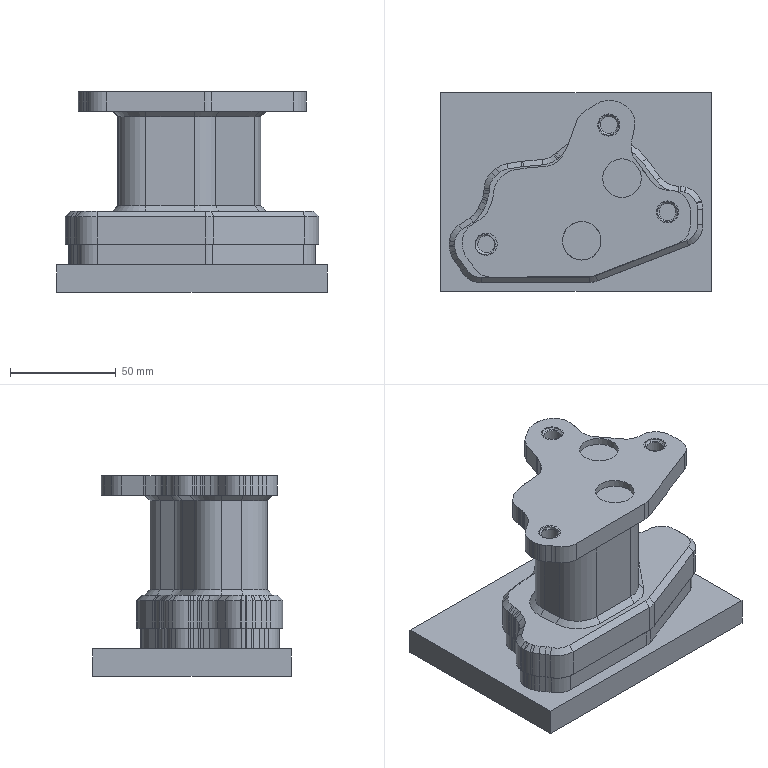NC program | NX | posted by the shop | part box 128.162 x 94.109 x 95 mm
Lines 1 to 907 of 131503:
1 BEGIN PGM A MM
2 BLK FORM 0.1 Z X-200 Y-200 Z-20
3 BLK FORM 0.2  X+200  Y+200  Z+0
4 CYCL DEF 247 DATUM SETTING ~
Q339=+1
5 * - OPERATION: 动态开粗_COPY - TOOL: T17 C-D20
6 M5
7 M9
8 PLANE RESET STAY
9 CALL LBL100
10 ;(C-D20 D=20. R=0.)
11 M01
12 TOOL CALL 17 Z S5500
13 CALL LBL101
14 M3 M8
15 M51
16 CYCL DEF 7.0
17 CYCL DEF 7.1 X0
18 CYCL DEF 7.2 Y0
19 CYCL DEF 7.3 Z0
20 CYCL DEF 32.0 TOLERANCE
21 CYCL DEF 32.1 T0.096
22 CYCL DEF 32.2 HSC-MODE:0
23 L M126
24 L A+0.0 C+0.0 FMAX
25 L X-64.6381 Y-62.2688 FMAX
26 L Z5.6 FMAX
27 L Z-41.4 FMAX
28 L Z-44.4 F4000.
29 L X-65.2249 Y-58.6321
30 CC X-67.2211 Y-58.9557
31 C X-66.6876 Y-57.005 DR+
32 CC X-63.5608 Y-44.6263
33 C X-75.0894 Y-50.1127 DR-
34 CC X-50.9463 Y-38.6348
35 C X-77.6301 Y-40.2486 DR-
36 CC X129.1158 Y-26.3608
37 C X-78.0747 Y-23.3848 DR-
38 L X-78.046 Y43.4708
39 CC X-66.5594 Y42.2154
40 C X-73.4593 Y51.4841 DR-
41 CC X-81.0452 Y57.4973
42 C X-72.4257 Y53.0917 DR+
43 CC X-63.9857 Y46.8105
44 C X-66.5375 Y57.0172 DR-
45 CC X-66.994 Y58.9644
46 C X-67.3023 Y60.9405 DR+
47 L X-67.7443 Y60.8715
48 L X-71.6615 Y60.2602 Z-43.9
49 L X-74.0482 Y59.8878 F15000.
50 CC X-73.7265 Y57.8856
51 C X-75.154 Y59.3259 DR+
52 L X-82.9516 Y51.5284
53 CC X-77.8446 Y46.4233
54 C X-85.0656 Y46.4246 DR+
55 L Y-25.4627
56 CC X15.891 Y-25.4556
57 C X-83.3393 Y-44.0456 DR+
58 L X-82.356 Y-49.2923
59 CC X-69.1974 Y-46.8244
60 C X-78.8027 Y-56.1505 DR+
61 L X-75.8842 Y-59.1556
62 CC X-74.4382 Y-57.7401
63 C X-74.7351 Y-59.7417 DR+
64 L X-71.9244 Y-60.1472
65 L X-70.0495 Y-60.4256 Z-44.1391 F4000.
66 L X-68.1703 Y-60.6737 Z-44.3782
67 L X-67.9978 Y-60.6835 Z-44.4
68 CC X-68.0574 Y-58.6844
69 C X-67.2677 Y-56.8468 DR+
70 CC X-63.9193 Y-46.8931
71 C X-73.873 Y-50.2416 DR-
72 CC X-32.3004 Y-34.5195
73 C X-76.7096 Y-36.3333 DR-
74 CC X259.3441 Y-20.2611
75 C X-77.0763 Y-16.8399 DR-
76 L X-77.0385 Y39.5418
77 CC X-57.875 Y37.4408
78 C X-74.5031 Y47.1958 DR-
79 CC X-93.6033 Y51.8201
80 C X-74.0913 Y49.4785 DR+
81 CC X-64.3957 Y46.985
82 C X-73.0825 Y51.9611 DR-
83 CC X-74.8273 Y52.9389
84 C X-74.8609 Y54.9387 DR+
85 CC X-74.7828 Y52.7966
86 CP IPA39.8769 IZ.1881 DR+
87 L X-78.155 Y52.8585 Z-43.9
88 L X-79.1315 Y52.0981 F15000.
89 L X-80.0829 Y51.3065
90 CC X-78.6074 Y49.9349
91 C X-80.6219 Y49.9409 DR+
92 L X-80.6327 Y-46.3389
93 CC X-78.5897 Y-46.3266
94 C X-80.3179 Y-47.4161 DR+
95 L X-79.1856 Y-49.188
96 L X-78.2717 Y-50.635 Z-44.116 F4000.
97 L X-77.3271 Y-52.0622 Z-44.3319
98 L X-76.9257 Y-52.4226 Z-44.4
99 CC X-75.8026 Y-50.7677
100 C X-73.873 Y-50.2416 DR+
101 CC X-55.3891 Y-45.2768
102 C X-74.4854 Y-46.5552 DR-
103 CC X78.9759 Y-24.6557
104 C X-76.0352 Y-23.4267 DR-
105 L X-76.0582 Y35.6979
106 CC X-44.9209 Y33.8344
107 C X-74.4274 Y43.9524 DR-
108 L X-74.3565 Y47.7592
109 CC X-76.3567 Y47.7861
110 C X-76.5758 Y49.7745 DR+
111 CC X-76.3099 Y47.6971
112 CP IPA51.5204 IZ.2375 DR+
113 L X-79.2965 Y47.0806 Z-43.9
114 L X-80.7527 Y45.0077 F15000.
115 CC X-79.0849 Y43.8481
116 C X-81.1162 Y43.8565 DR+
117 L X-81.0479 Y-44.3701
118 CC X-79.0136 Y-44.3579
119 C X-80.6972 Y-45.4998 DR+
120 L X-79.3207 Y-47.5066
121 L X-78.5503 Y-48.6479 Z-44.0738 F4000.
122 L X-77.7443 Y-49.7644 Z-44.2477
123 CC X-76.2434 Y-48.3254
124 CP IPA33.3004 IZ-.1523 DR+
125 CC X-76.2845 Y-48.3972
126 C X-74.2882 Y-48.2728 DR+
127 CC X26.3005 Y-43.293
128 C X-74.3991 Y-41.7213 DR-
129 CC X483.5474 Y-13.8433
130 C X-75.0754 Y-9.1457 DR-
131 L X-75.0405 Y33.1679
132 CC X-28.9846 Y30.8517
133 C X-74.3801 Y38.9614 DR-
134 L Y44.3364
135 CC X-76.3801 Y44.3363
136 C X-78.2435 Y45.0628 DR+
137 L X-79.3058 Y41.2435 Z-43.9
138 L X-79.609 Y40.1683 F15000.
139 L X-79.8813 Y39.0849
140 L X-79.8993 Y38.8171
141 L Y-36.9087
142 L X-79.8276 Y-37.4395
143 L X-79.343 Y-39.1999
144 L X-78.2898 Y-43.022 Z-44.4 F4000.
145 CC X-76.3801 Y-42.4279
146 C X-74.3801 Y-42.428 DR+
147 L Y39.072
148 CC X-76.401 Y39.0713
149 C X-76.0188 Y41.0557 DR+
150 L X-79.1882 Y41.6649
151 CC X-79.5695 Y39.6812
152 C X-79.3149 Y37.6773 DR+
153 L Z-41.4
154 L Z5.6 FMAX
155 L X-64.6381 Y-62.2688 FMAX
156 L Z-78.7 FMAX
157 L Z-81.7
158 L X-65.2249 Y-58.6321
159 CC X-67.2211 Y-58.9557
160 C X-66.6876 Y-57.005 DR+
161 CC X-63.5608 Y-44.6263
162 C X-75.0894 Y-50.1127 DR-
163 CC X-50.9463 Y-38.6348
164 C X-77.6301 Y-40.2486 DR-
165 CC X129.1158 Y-26.3608
166 C X-78.0747 Y-23.3848 DR-
167 L X-78.046 Y43.4708
168 CC X-66.5594 Y42.2154
169 C X-73.4593 Y51.4841 DR-
170 CC X-81.0452 Y57.4973
171 C X-72.4257 Y53.0917 DR+
172 CC X-63.9857 Y46.8105
173 C X-66.5375 Y57.0172 DR-
174 CC X-66.994 Y58.9644
175 C X-67.3023 Y60.9405 DR+
176 L X-67.7443 Y60.8715
177 L X-71.6615 Y60.2602 Z-81.2
178 L X-74.0482 Y59.8878 F15000.
179 CC X-73.7265 Y57.8856
180 C X-75.154 Y59.3259 DR+
181 L X-82.9516 Y51.5284
182 CC X-77.8446 Y46.4233
183 C X-85.0656 Y46.4246 DR+
184 L Y-25.4627
185 CC X15.891 Y-25.4556
186 C X-83.3393 Y-44.0456 DR+
187 L X-82.356 Y-49.2923
188 CC X-69.1974 Y-46.8244
189 C X-78.8027 Y-56.1505 DR+
190 L X-75.8842 Y-59.1556
191 CC X-74.4382 Y-57.7401
192 C X-74.7351 Y-59.7417 DR+
193 L X-71.9244 Y-60.1472
194 L X-70.0495 Y-60.4256 Z-81.4391 F4000.
195 L X-68.1703 Y-60.6737 Z-81.6782
196 L X-67.9978 Y-60.6835 Z-81.7
197 CC X-68.0574 Y-58.6844
198 C X-67.2677 Y-56.8468 DR+
199 CC X-63.9193 Y-46.8931
200 C X-73.873 Y-50.2416 DR-
201 CC X-32.3004 Y-34.5195
202 C X-76.7096 Y-36.3333 DR-
203 CC X259.3441 Y-20.2611
204 C X-77.0763 Y-16.8399 DR-
205 L X-77.0385 Y39.5418
206 CC X-57.875 Y37.4408
207 C X-74.5031 Y47.1958 DR-
208 CC X-93.6033 Y51.8201
209 C X-74.0913 Y49.4785 DR+
210 CC X-64.3957 Y46.985
211 C X-73.0825 Y51.9611 DR-
212 CC X-74.8273 Y52.9389
213 C X-74.8609 Y54.9387 DR+
214 CC X-74.7828 Y52.7966
215 CP IPA39.8769 IZ.1881 DR+
216 L X-78.155 Y52.8585 Z-81.2
217 L X-79.1315 Y52.0981 F15000.
218 L X-80.0829 Y51.3065
219 CC X-78.6074 Y49.9349
220 C X-80.6219 Y49.9409 DR+
221 L X-80.6327 Y-46.3389
222 CC X-78.5897 Y-46.3266
223 C X-80.3179 Y-47.4161 DR+
224 L X-79.1856 Y-49.188
225 L X-78.2717 Y-50.635 Z-81.416 F4000.
226 L X-77.3271 Y-52.0622 Z-81.6319
227 L X-76.9257 Y-52.4226 Z-81.7
228 CC X-75.8026 Y-50.7677
229 C X-73.873 Y-50.2416 DR+
230 CC X-55.3891 Y-45.2768
231 C X-74.4854 Y-46.5552 DR-
232 CC X78.9759 Y-24.6557
233 C X-76.0352 Y-23.4267 DR-
234 L X-76.0582 Y35.6979
235 CC X-44.9209 Y33.8344
236 C X-74.4274 Y43.9524 DR-
237 L X-74.3565 Y47.7592
238 CC X-76.3567 Y47.7861
239 C X-76.5758 Y49.7745 DR+
240 CC X-76.3099 Y47.6971
241 CP IPA51.5204 IZ.2375 DR+
242 L X-79.2965 Y47.0806 Z-81.2
243 L X-80.7527 Y45.0077 F15000.
244 CC X-79.0849 Y43.8481
245 C X-81.1162 Y43.8565 DR+
246 L X-81.0479 Y-44.3701
247 CC X-79.0136 Y-44.3579
248 C X-80.6972 Y-45.4998 DR+
249 L X-79.3207 Y-47.5066
250 L X-78.5503 Y-48.6479 Z-81.3738 F4000.
251 L X-77.7443 Y-49.7644 Z-81.5477
252 CC X-76.2434 Y-48.3254
253 CP IPA33.3004 IZ-.1523 DR+
254 CC X-76.2845 Y-48.3972
255 C X-74.2882 Y-48.2728 DR+
256 CC X26.3006 Y-43.293
257 C X-74.3991 Y-41.7213 DR-
258 CC X483.5474 Y-13.8433
259 C X-75.0754 Y-9.1457 DR-
260 L X-75.0405 Y33.1679
261 CC X-28.9846 Y30.8517
262 C X-74.3801 Y38.9614 DR-
263 L Y44.3364
264 CC X-76.3801 Y44.3363
265 C X-78.2435 Y45.0628 DR+
266 L X-79.3058 Y41.2435 Z-81.2
267 L X-79.609 Y40.1683 F15000.
268 L X-79.8813 Y39.0849
269 L X-79.8993 Y38.8171
270 L Y-36.9087
271 L X-79.8276 Y-37.4395
272 L X-79.343 Y-39.1999
273 L X-78.2898 Y-43.022 Z-81.7 F4000.
274 CC X-76.3801 Y-42.4279
275 C X-74.3801 Y-42.428 DR+
276 L Y39.072
277 CC X-76.401 Y39.0713
278 C X-76.0188 Y41.0557 DR+
279 L X-79.1882 Y41.6649
280 CC X-79.5695 Y39.6812
281 C X-79.3149 Y37.6773 DR+
282 L Z-78.7
283 L Z5.6 FMAX
284 L X62.5938 Y62.3089 FMAX
285 L Z-41.4 FMAX
286 L Z-44.4
287 CC X62.6738 Y60.2896
288 C X64.6499 Y60.7124 DR-
289 L X65.1088 Y58.5642
290 CC X67.0859 Y58.9878
291 C X66.7119 Y57.0007 DR+
292 CC X63.4656 Y44.5388
293 C X75.1287 Y49.9985 DR-
294 CC X50.4575 Y38.4647
295 C X77.6487 Y39.9932 DR-
296 CC X-132.8635 Y26.3435
297 C X78.0733 Y23.6284 DR-
298 L X78.0464 Y-43.4545
299 CC X66.5542 Y-42.2325
300 C X73.4839 Y-51.4815 DR-
301 L X71.9663 Y-53.6802
302 CC X62.8803 Y-45.5088
303 C X68.5579 Y-56.3297 DR-
304 L X66.7172 Y-57.0079
305 CC X67.2019 Y-58.9502
306 C X67.6274 Y-60.9064 DR+
307 L X71.5448 Y-60.2964 Z-43.9
308 L X74.2272 Y-59.8787 F15000.
309 CC X73.9063 Y-57.8764
310 C X75.3337 Y-59.3167 DR+
311 L X83.1313 Y-51.5192
312 CC X78.0243 Y-46.4141
313 C X85.2453 Y-46.4154 DR+
314 L Y25.5025
315 CC X-12.8027 Y25.4957
316 C X83.4802 Y44.0164 DR+
317 L X82.4553 Y49.3429
318 CC X70.0761 Y46.9591
319 C X78.925 Y55.9381 DR+
320 L X75.572 Y59.2417
321 CC X74.1549 Y57.7902
322 C X74.4684 Y59.7944 DR+
323 L X71.7716 Y60.2035
324 L X67.8514 Y60.7952 Z-44.4 F4000.
325 CC X67.661 Y58.8043
326 C X66.9555 Y56.9329 DR+
327 CC X63.9621 Y46.9025
328 C X73.7629 Y50.5783 DR-
329 CC X31.4752 Y34.3855
330 C X76.7259 Y36.0708 DR-
331 CC X-272.8684 Y20.0983
332 C X77.0752 Y16.8268 DR-
333 L X77.0473 Y-39.4006
334 CC X57.7068 Y-37.4513
335 C X74.4658 Y-47.2998 DR-
336 CC X79.0145 Y-48.6425
337 C X74.2732 Y-48.5223 DR+
338 CC X63.5123 Y-46.8644
339 C X73.1423 Y-51.9446 DR-
340 CC X74.9604 Y-52.7786
341 C X74.7473 Y-54.7674 DR+
342 CC X74.9365 Y-52.6722
343 CP IPA46.4743 IZ.2151 DR+
344 L X78.1168 Y-52.8805 Z-43.9
345 L X79.1344 Y-52.1132 F15000.
346 L X80.1259 Y-51.3124
347 CC X78.6684 Y-49.9233
348 C X80.6818 Y-49.9244 DR+
349 L X80.4755 Y46.7914
350 CC X78.4306 Y46.7741
351 C X80.1648 Y47.8577 DR+
352 L X79.1147 Y49.5148
353 L X77.2267 Y52.4725 Z-44.3428 F4000.
354 L X76.9202 Y52.8069 Z-44.4
355 CC X75.628 Y51.2803
356 C X73.7158 Y50.6941 DR+
357 CC X56.9761 Y45.3618
358 C X74.5117 Y46.4364 DR-
359 CC X-82.3019 Y24.4596
360 C X76.0379 Y23.0517 DR-
361 L X76.0526 Y-35.8229
362 CC X44.5148 Y-33.7783
363 C X74.415 Y-44.015 DR-
364 L X74.3105 Y-47.9258
365 CC X76.3069 Y-48.0502
366 C X76.664 Y-50.0183 DR+
367 CC X76.2558 Y-47.9616
368 CP IPA48.1212 IZ.222 DR+
369 L X79.305 Y-47.2152 Z-43.9
370 L X80.1055 Y-46.0667 F15000.
371 L X80.8701 Y-44.894
372 L X81.0159 Y-44.469
373 L X81.0702 Y-44.0231
374 L X81.1135 Y43.8565
375 CC X79.082 Y43.8475
376 C X80.7506 Y45.0063 DR+
377 L X79.3324 Y47.0274
378 L X77.8867 Y49.0644 Z-44.2154 F4000.
379 CC X76.3416 Y47.788
380 CP IPA41.8361 IZ-.1846 DR+
381 CC X76.3539 Y47.7901
382 C X74.3538 Y47.7592 DR+
383 CC X359.4998 Y48.4494
384 C X74.8188 Y32.1579 DR+
385 CC X-816.6851 Y9.671
386 C X75.0767 Y2.9105 DR-
387 L X75.0408 Y-33.1515
388 CC X31.263 Y-31.0727
389 C X74.3807 Y-38.9263 DR-
390 L Y-44.3013
391 CC X76.3807 Y-44.3013
392 C X78.2705 Y-44.9561 DR+
393 L X79.3267 Y-41.1348 Z-43.9
394 L X79.6191 Y-40.0963 F15000.
395 L X79.8819 Y-39.0499
396 L X79.8999 Y-38.7821
397 L Y36.8956
398 L X79.8282 Y37.4264
399 L X79.3211 Y39.2688
400 L X78.2634 Y43.0896 Z-44.4 F4000.
401 CC X76.3807 Y42.4148
402 C X74.3807 Y42.4149 DR+
403 L Y-38.9601
404 CC X76.401 Y-38.9598
405 C X76.6988 Y-40.958 DR+
406 L X79.3347 Y-40.5647
407 L Z-41.4
408 L Z5.6 FMAX
409 L X62.5938 Y62.3089 FMAX
410 L Z-78.7 FMAX
411 L Z-81.7
412 CC X62.6738 Y60.2896
413 C X64.6474 Y60.724 DR-
414 L X65.125 Y58.55
415 CC X67.0998 Y58.9853
416 C X66.7119 Y57.0007 DR+
417 CC X63.4656 Y44.5388
418 C X75.1287 Y49.9985 DR-
419 CC X50.4575 Y38.4647
420 C X77.6487 Y39.9932 DR-
421 CC X-132.8635 Y26.3435
422 C X78.0733 Y23.6284 DR-
423 L X78.0464 Y-43.4545
424 CC X66.5542 Y-42.2325
425 C X73.4839 Y-51.4815 DR-
426 L X71.9663 Y-53.6802
427 CC X62.8803 Y-45.5088
428 C X68.5579 Y-56.3297 DR-
429 L X66.7172 Y-57.0079
430 CC X67.2019 Y-58.9502
431 C X67.6274 Y-60.9064 DR+
432 L X71.5448 Y-60.2964 Z-81.2
433 L X74.2272 Y-59.8787 F15000.
434 CC X73.9063 Y-57.8764
435 C X75.3337 Y-59.3167 DR+
436 L X83.1313 Y-51.5192
437 CC X78.0243 Y-46.4141
438 C X85.2453 Y-46.4154 DR+
439 L Y25.5025
440 CC X-12.8027 Y25.4957
441 C X83.4802 Y44.0164 DR+
442 L X82.4553 Y49.3429
443 CC X70.0761 Y46.9591
444 C X78.925 Y55.9381 DR+
445 L X75.572 Y59.2417
446 CC X74.1549 Y57.7902
447 C X74.4684 Y59.7944 DR+
448 L X71.7716 Y60.2035
449 L X67.8514 Y60.7952 Z-81.7 F4000.
450 CC X67.661 Y58.8043
451 C X66.9555 Y56.9329 DR+
452 CC X63.9621 Y46.9025
453 C X73.7629 Y50.5783 DR-
454 CC X31.4752 Y34.3855
455 C X76.7259 Y36.0708 DR-
456 CC X-272.8684 Y20.0983
457 C X77.0752 Y16.8268 DR-
458 L X77.0473 Y-39.4006
459 CC X57.7068 Y-37.4513
460 C X74.4658 Y-47.2998 DR-
461 CC X79.0145 Y-48.6425
462 C X74.2732 Y-48.5223 DR+
463 CC X63.5123 Y-46.8644
464 C X73.1423 Y-51.9446 DR-
465 CC X74.9604 Y-52.7786
466 C X74.7473 Y-54.7674 DR+
467 CC X74.9365 Y-52.6722
468 CP IPA46.4743 IZ.2151 DR+
469 L X78.1168 Y-52.8805 Z-81.2
470 L X79.1344 Y-52.1132 F15000.
471 L X80.1259 Y-51.3124
472 CC X78.6684 Y-49.9233
473 C X80.6818 Y-49.9244 DR+
474 L X80.4755 Y46.7914
475 CC X78.4306 Y46.7741
476 C X80.1648 Y47.8577 DR+
477 L X79.1147 Y49.5148
478 L X77.2267 Y52.4725 Z-81.6428 F4000.
479 L X76.9202 Y52.8069 Z-81.7
480 CC X75.628 Y51.2803
481 C X73.7158 Y50.6941 DR+
482 CC X56.9761 Y45.3618
483 C X74.5117 Y46.4364 DR-
484 CC X-82.3019 Y24.4596
485 C X76.0379 Y23.0517 DR-
486 L X76.0526 Y-35.8229
487 CC X44.5148 Y-33.7783
488 C X74.415 Y-44.015 DR-
489 L X74.3105 Y-47.9258
490 CC X76.3069 Y-48.0502
491 C X76.664 Y-50.0183 DR+
492 CC X76.2558 Y-47.9616
493 CP IPA48.1212 IZ.222 DR+
494 L X79.305 Y-47.2152 Z-81.2
495 L X80.1055 Y-46.0667 F15000.
496 L X80.8701 Y-44.894
497 L X81.0159 Y-44.469
498 L X81.0702 Y-44.0231
499 L X81.1135 Y43.8565
500 CC X79.082 Y43.8475
501 C X80.7506 Y45.0063 DR+
502 L X79.3324 Y47.0274
503 L X77.8867 Y49.0644 Z-81.5154 F4000.
504 CC X76.3416 Y47.788
505 CP IPA41.8361 IZ-.1846 DR+
506 CC X76.3539 Y47.7901
507 C X74.3538 Y47.7592 DR+
508 CC X359.4999 Y48.4494
509 C X74.8188 Y32.1579 DR+
510 CC X-816.6851 Y9.671
511 C X75.0767 Y2.9105 DR-
512 L X75.0408 Y-33.1515
513 CC X31.263 Y-31.0727
514 C X74.3807 Y-38.9263 DR-
515 L Y-44.3013
516 CC X76.3807 Y-44.3013
517 C X78.2705 Y-44.9561 DR+
518 L X79.3267 Y-41.1348 Z-81.2
519 L X79.6191 Y-40.0963 F15000.
520 L X79.8819 Y-39.0499
521 L X79.8999 Y-38.7821
522 L Y36.8956
523 L X79.8282 Y37.4264
524 L X79.3211 Y39.2688
525 L X78.2634 Y43.0896 Z-81.7 F4000.
526 CC X76.3807 Y42.4148
527 C X74.3807 Y42.4149 DR+
528 L Y-38.9601
529 CC X76.401 Y-38.9598
530 C X76.6988 Y-40.958 DR+
531 L X79.3347 Y-40.5647
532 L Z-78.7
533 L Z5.6 FMAX
534 PLANE RESET STAY
535 * - OPERATION: 精飞平面 - TOOL: T17 C-D20
536 CYCL DEF 32.0 TOLERANCE
537 CYCL DEF 32.1 T0.036
538 CYCL DEF 32.2 HSC-MODE:0
539 L A+0.0 C+0.0 FMAX
540 L X76.2809 Y-40.7534 FMAX
541 L Z43. FMAX
542 L Z3.1 FMAX
543 L Z.1 F1500.
544 L X74.0809
545 L X-74.0809
546 L Y-24.452
547 L X74.0809
548 L Y-8.1507
549 L X-74.0809
550 L Y8.1507
551 L X74.0809
552 L Y24.452
553 L X-74.0809
554 L Y40.7534
555 L X74.0809
556 L X76.2809
557 L Z3.1
558 L Z43. FMAX
559 PLANE RESET STAY
560 * - OPERATION: 动态开粗 - TOOL: T17 C-D20
561 CYCL DEF 32.0 TOLERANCE
562 CYCL DEF 32.1 T0.096
563 CYCL DEF 32.2 HSC-MODE:0
564 L A+0.0 C+0.0 FMAX
565 L X-79.1931 Y-24.9744 FMAX
566 L Z5.6 FMAX
567 L Z-41.4 FMAX
568 L Z-44.4 F4000.
569 L X-76.8858 Y-26.1193
570 CC X-75.9882 Y-24.3093
571 C X-74.0804 Y-24.9744 DR+
572 CC X-103.6147 Y-17.8744
573 C X-73.2393 Y-17.7376 DR+
574 CC X-767.6787 Y-2.7045
575 C X-73.0802 Y-.4558 DR+
576 L X-73.0461 Y43.4708
577 CC X-61.3176 Y42.1555
578 C X-67.363 Y52.2917 DR-
579 CC X-55.5707 Y32.5157
580 C X-57.5748 Y55.4532 DR-
581 CC X-45.0783 Y-76.5411
582 C X-43.3441 Y56.0321 DR-
583 L X60.4448 Y56.0206
584 CC X59.2035 Y44.4007
585 C X69.1338 Y50.5612 DR-
586 CC X49.7352 Y38.5467
587 C X72.4633 Y40.5691 DR-
588 CC X-57.4553 Y27.9966
589 C X73.058 Y26.2144 DR-
590 L X73.0458 Y-43.4545
591 CC X61.4086 Y-42.1991
592 C X67.4768 Y-52.208 DR-
593 CC X55.6256 Y-32.7006
594 C X57.71 Y-55.4305 DR-
595 CC X45.0627 Y74.1115
596 C X43.2308 Y-56.0335 DR-
597 L X-60.6053 Y-56.014
598 CC X-59.2123 Y-44.3836
599 C X-69.1658 Y-50.5589 DR-
600 CC X-49.87 Y-38.6409
601 C X-72.4571 Y-40.6881 DR-
602 CC X8.786 Y-31.2452
603 C X-72.5692 Y-22.822 DR-
604 CC X-387.5348 Y-5.2348
605 C X-72.0878 Y-2.8148 DR+
606 L X-72.0491 Y39.4175
607 CC X-57.4642 Y38.2757
608 C X-64.4942 Y51.1054 DR-
609 CC X-51.0693 Y26.4223
610 C X-53.3108 Y54.4305 DR-
611 CC X-39.0488 Y-108.9859
612 C X-36.8296 Y55.0367 DR-
613 L X56.3912 Y55.0229
614 CC X55.2639 Y40.4088
615 C X68.1102 Y47.467 DR-
616 CC X43.4345 Y34.0086
617 C X71.4496 Y36.2827 DR-
618 CC X-79.1815 Y22.6646
619 C X72.0553 Y21.0518 DR-
620 L X72.0402 Y-39.5255
621 CC X57.4537 Y-38.2618
622 C X64.4734 Y-51.1104 DR-
623 CC X51.0351 Y-26.3439
624 C X53.2772 Y-54.4319 DR-
625 CC X39.2625 Y104.7801
626 C X37.296 Y-55.0355 DR-
627 L X-56.4266 Y-55.0241
628 CC X-55.2981 Y-40.4413
629 C X-68.1338 Y-47.4539 DR-
630 CC X-43.8328 Y-34.1812
631 C X-71.4123 Y-36.6461 DR-
632 CC X-4.493 Y-29.5245
633 C X-71.6233 Y-24.7892 DR-
634 CC X-660.7992 Y1.1722
635 C X-71.0761 Y6.5373 DR+
636 L X-71.0451 Y36.0373
637 CC X-54.4393 Y35.2875
638 C X-61.8862 Y50.1488 DR-
639 CC X-47.5727 Y21.3661
640 C X-50.0248 Y53.4178 DR-
641 CC X-35.091 Y-123.7813
642 C X-33.043 Y54.0341 DR-
643 L X52.8317 Y54.0264
644 CC X52.2865 Y37.3989
645 C X67.1224 Y44.9265 DR-
646 CC X38.5947 Y30.5765
647 C X70.4302 Y33.0774 DR-
648 CC X-112.4859 Y17.634
649 C X71.0634 Y15.0964 DR-
650 L X71.0493 Y-35.9032
651 CC X54.4523 Y-35.2873
652 C X61.981 Y-50.0913 DR-
653 CC X47.7926 Y-22.0839
654 C X50.5122 Y-53.3622 DR-
655 CC X35.214 Y116.0301
656 C X32.9087 Y-54.036 DR-
657 L X-53.0907 Y-54.0172
658 CC X-52.3018 Y-37.4024
659 C X-67.1863 Y-44.8272 DR-
660 CC X-39.488 Y-31.0006
661 C X-70.427 Y-32.0735 DR-
662 CC X93.5889 Y-26.2135
663 C X-70.3363 Y-18.2102 DR-
664 CC X-979.1699 Y4.5471
665 C X-70.0784 Y11.5402 DR+
666 CC X878.9921 Y19.8935
667 C X-70.017 Y33.542 DR-
668 CC X-51.896 Y32.7543
669 C X-59.6515 Y49.1507 DR-
670 CC X-44.5708 Y16.9764
671 C X-47.1445 Y52.4163 DR-
672 CC X-31.3648 Y-144.4649
673 C X-29.1619 Y53.0354 DR-
674 L X11.9637 Y53.0668
675 CC X16.3169 Y22.3388
676 C X19.2858 Y53.2313 DR-
677 CC X39.7258 Y1015.9654
678 C X48.0157 Y53.0501 DR+
679 CC X49.0523 Y32.1833
680 C X58.0821 Y51.0237 DR-
681 CC X48.7082 Y33.83
682 C X67.1145 Y40.5158 DR-
683 CC X26.0842 Y25.7234
684 C X69.6606 Y27.5658 DR-
685 CC X-312.1338 Y9.0746
686 C X70.0754 Y4.0737 DR-
687 L X70.0352 Y-33.1511
688 CC X51.8548 Y-32.7196
689 C X59.5761 Y-49.1846 DR-
690 CC X44.6091 Y-17.0786
691 C X47.301 Y-52.3994 DR-
692 CC X31.8843 Y132.6011
693 C X30.0693 Y-53.0318 DR-
694 L X-49.9274 Y-53.0206
695 CC X-49.7066 Y-34.7688
696 C X-66.3742 Y-42.2099 DR-
697 CC X-36.1997 Y-28.7343
698 C X-69.2273 Y-29.8595 DR-
699 CC X133.6335 Y-22.0111
700 C X-69.2465 Y-14.6742 DR-
701 CC X-1025.6017 Y4.9783
702 C X-69.0744 Y12.5366 DR+
703 CC X521.0636 Y19.29
704 C X-68.9911 Y31.2855 DR-
705 CC X-49.6782 Y30.5206
706 C X-57.8073 Y48.056 DR-
707 CC X-42.2199 Y14.1798
708 C X-45.1736 Y51.3529 DR-
709 CC X-28.4949 Y-148.0887
710 C X-26.0686 Y52.0344 DR-
711 L X7.8899 Y52.0739
712 CC X15.9792 Y27.7752
713 C X21.8989 Y52.6915 DR-
714 CC X33.1331 Y154.3707
715 C X34.7141 Y52.085 DR+
716 CC X38.0217 Y-295.1394
717 C X48.6442 Y51.9382 DR-
718 CC X47.5309 Y32.6196
719 C X65.1328 Y40.6585 DR-
720 CC X31.1758 Y25.1909
721 C X68.3639 Y28.2506 DR-
722 CC X-125.9894 Y11.6332
723 C X69.0588 Y9.2714 DR-
724 L X69.0487 Y-29.9783
725 CC X49.0081 Y-30.2354
726 C X64.8348 Y-42.5321 DR-
727 CC X47.435 Y-27.7197
728 C X53.3926 Y-49.7803 DR-
729 CC X38.1987 Y6.6141
730 C X39.4451 Y-51.7779 DR-
731 CC X20.2114 Y574.5371
732 C X14.9486 Y-52.051 DR-
733 L X-47.1761 Y-52.0192
734 CC X-47.3409 Y-32.2541
735 C X-60.274 Y-47.2015 DR-
736 CC X-44.5143 Y-30.4719
737 C X-66.9994 Y-35.2326 DR-
738 CC X-8.5947 Y-22.9533
739 C X-68.2655 Y-21.822 DR-
740 L X-68.0769 Y9.0483
741 CC X657.1293 Y15.8438
742 C X-67.9932 Y28.7917 DR-
743 CC X-47.5571 Y28.4043
744 C X-55.8405 Y47.0903 DR-
745 CC X-39.7648 Y10.5572
746 C X-42.8057 Y50.3548 DR-
747 CC X-25.1363 Y-171.8932
748 C X-22.2 Y51.0367 DR-
749 L X5.0633 Y51.0775
750 CC X4.7996 Y55.747
751 C X7.2432 Y51.7593 DR+
752 CC X12.7872 Y39.9081
753 C X10.6802 Y52.8211 DR-
754 L X12.4045 Y53.1495
755 CC X15.4854 Y30.3956
756 C X15.8431 Y53.3543 DR-
757 CC X16.2034 Y24.2804
758 C X19.2817 Y53.1932 DR-
759 CC X4.298 Y-23.1029
760 C X24.6658 Y51.9354 DR-
761 CC X35.4039 Y123.4693
762 C X35.9322 Y51.1359 DR+
763 CC X37.1619 Y-135.8876
764 C X47.0689 Y50.8774 DR-
765 CC X45.5095 Y30.6187
766 C X64.0193 Y38.9991 DR-
767 CC X28.4715 Y22.9741
768 C X67.328 Y26.2337 DR-
769 CC X-130.2771 Y9.0898
770 C X68.0565 Y6.7558 DR-
771 L X68.0503 Y-27.2766
772 CC X44.9804 Y-27.6813
773 C X65.3216 Y-38.5725 DR-
774 CC X46.5871 Y-27.3374
775 C X53.7818 Y-47.9638 DR-
776 CC X38.001 Y-2.6063
777 C X40.3297 Y-50.5741 DR-
778 CC X22.5364 Y272.2534
779 C X19.0892 Y-51.0457 DR-
780 L X-44.8027 Y-51.011
781 CC X-45.0324 Y-29.3289
782 C X-57.1793 Y-47.2905 DR-
783 CC X-43.8297 Y-29.4254
784 C X-65.3917 Y-35.1221 DR-
785 CC X-13.6363 Y-21.5389
786 C X-67.1443 Y-21.3984 DR-
787 CC X931.6977 Y-11.8259
788 C X-67.0883 Y2.4395 DR-
789 L X-67.033 Y25.5447
790 CC X-42.9122 Y25.7124
791 C X-64.0717 Y37.2931 DR-
792 CC X-44.7192 Y25.4395
793 C X-52.1104 Y46.8964 DR-
794 CC X-35.8548 Y-.3177
795 C X-38.2831 Y49.5573 DR-
796 CC X-19.6209 Y-291.8834
797 C X-15.6679 Y50.0441 DR-
798 CC X-9.1908 Y865.0086
799 C X3.0362 Y50.1101 DR+
800 CC X2.9206 Y54.4963
801 C X5.5273 Y50.9668 DR+
802 CC X14.8927 Y33.3841
803 C X12.4045 Y53.1495 DR-
804 CC X15.4854 Y30.3956
805 C X15.8431 Y53.3543 DR-
806 CC X16.2034 Y24.2804
807 C X19.2817 Y53.1932 DR-
808 CC X16.1462 Y30.6982
809 C X25.243 Y51.5093 DR-
810 CC X34.811 Y88.7469
811 C X34.335 Y50.3027 DR+
812 CC X27.9591 Y-256.8808
813 C X44.9517 Y49.8986 DR-
814 CC X43.5219 Y28.6496
815 C X63.047 Y37.1546 DR-
816 CC X25.2034 Y20.7212
817 C X66.3209 Y24.1182 DR-
818 CC X-132.9521 Y6.9399
819 C X67.0507 Y5.0149 DR-
820 L X67.0396 Y-25.2347
821 CC X42.1692 Y-25.5406
822 C X64.4002 Y-36.6947 DR-
823 CC X44.9576 Y-25.7352
824 C X52.604 Y-46.7032 DR-
825 CC X36.2885 Y-1.8815
826 C X38.9317 Y-49.5071 DR-
827 CC X20.6528 Y250.5199
828 C X17.1936 Y-50.0435 DR-
829 L X10.0251 Y-50.0748
830 CC X5.5372 Y-30.0926
831 C X5.5273 Y-50.5726 DR-
832 L X-40.8942 Y-50.7472
833 CC X-38.4651 Y-12.0939
834 C X-51.1196 Y-48.6978 DR-
835 CC X-43.2303 Y-28.8063
836 C X-63.2795 Y-36.2856 DR-
837 CC X-22.8629 Y-21.3879
838 C X-65.913 Y-22.8489 DR-
839 CC X175.9639 Y-11.874
840 C X-66.1474 Y-9.2283 DR-
841 L X-66.029 Y23.4175
842 CC X-39.6961 Y23.5734
843 C X-63.4629 Y34.913 DR-
844 CC X-43.379 Y24.163
845 C X-51.4915 Y45.4494 DR-
846 CC X-34.7896 Y1.5291
847 C X-37.8612 Y48.4174 DR-
848 CC X-20.0447 Y-204.2159
849 C X-17.6265 Y49.0334 DR-
850 CC X-12.3648 Y841.966
851 C X.941 Y49.1275 DR+
852 CC X1.1502 Y53.6288
853 C X3.8751 Y50.04 DR+
854 CC X19.4244 Y23.7087
855 C X8.9659 Y52.4443 DR-
856 L X12.4045 Y53.1495
857 CC X15.4854 Y30.3956
858 C X15.8431 Y53.3543 DR-
859 CC X16.2034 Y24.2804
860 C X19.2817 Y53.1932 DR-
861 CC X16.1172 Y30.8096
862 C X26.4699 Y50.9059 DR-
863 CC X35.779 Y79.6854
864 C X34.8062 Y49.4534 DR+
865 CC X29.963 Y-88.1224
866 C X44.5458 Y48.764 DR-
867 CC X41.709 Y26.8838
868 C X61.956 Y35.6502 DR-
869 CC X22.9305 Y18.801
870 C X65.2877 Y22.3723 DR-
871 CC X-146.9963 Y4.1334
872 C X66.0553 Y1.6453 DR-
873 L X66.0429 Y-22.7766
874 CC X37.7087 Y-23.1952
875 C X64.0017 Y-33.7631 DR-
876 CC X43.6238 Y-24.4579
877 C X51.9278 Y-45.2639 DR-
878 CC X34.9737 Y-2.5523
879 C X37.962 Y-48.4085 DR-
880 CC X19.2716 Y219.0748
881 C X16.3552 Y-49.0448 DR-
882 CC X15.2875 Y-67.2674
883 C X13.204 Y-49.1329 DR+
884 CC X3.4282 Y-21.9544
885 C X9.9531 Y-50.0909 DR-
886 CC X10.3882 Y-52.0433
887 C X8.5075 Y-52.7247 DR+
888 CC X10.4649 Y-51.9763
889 CP IPA51.1433 IZ.2359 DR+
890 L X11.7608 Y-54.7486 Z-43.9
891 L X13.7532 Y-55.5568 F15000.
892 L X15.7577 Y-56.3343
893 L X16.2608 Y-56.3986
894 L X21.0372 Y-56.4043
895 L X25.8134 Y-56.3736
896 CC X23.6704 Y33.6762
897 C X38.4608 Y-55.1765 DR+
898 CC X23.726 Y41.9247
899 C X44.787 Y-54.0033 DR+
900 CC X31.5677 Y4.8252
901 C X53.1601 Y-51.4715 DR+
902 CC X37.0841 Y-11.1365
903 C X59.4677 Y-48.343 DR+
904 L X62.2797 Y-46.623
905 CC X53.109 Y-33.3929
906 C X67.9054 Y-39.7336 DR+